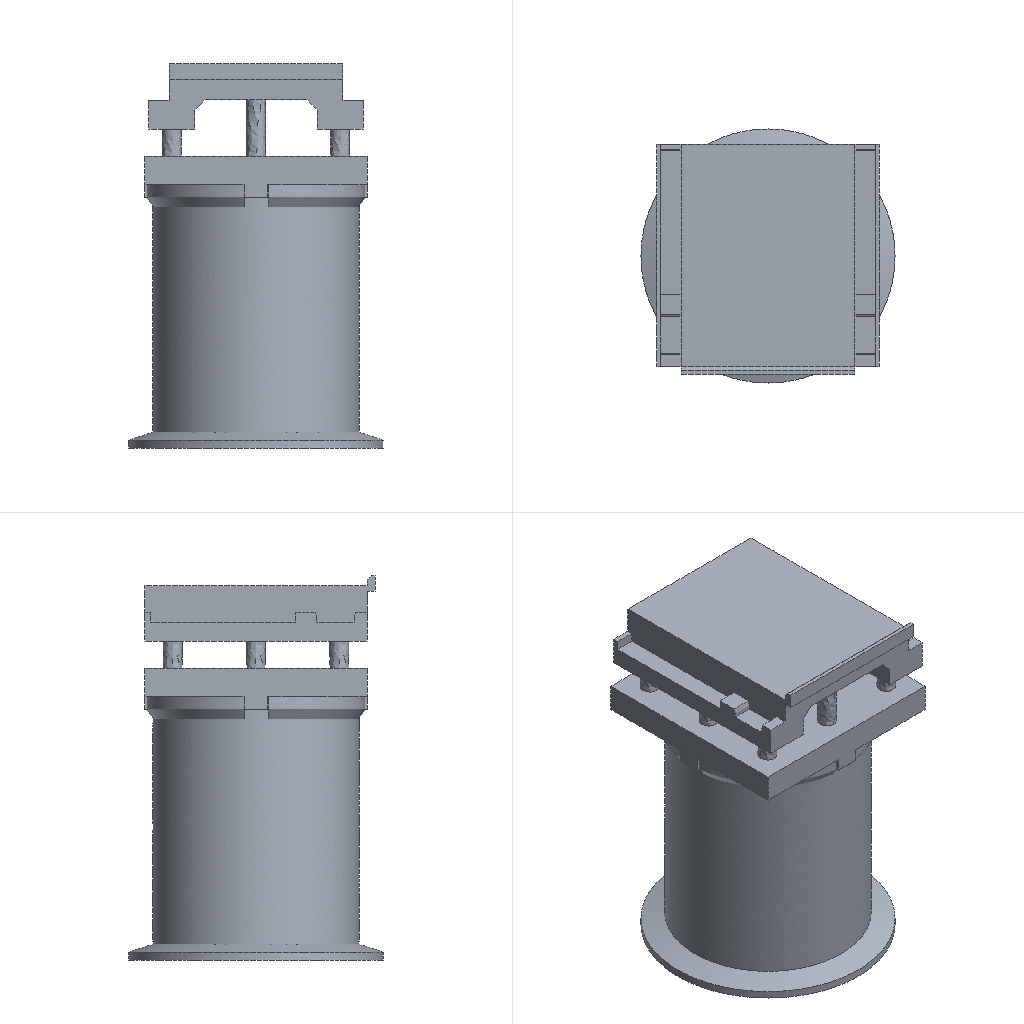Simulation study | ansys workbench
Ansys APDL input file, long lists of numbers shortened:
/batch
/config,noeldb,1     ! force off writing results to database
*get,_wallstrt,active,,time,wall
! ANSYS input file written by Workbench version 2022 R1
! File used for geometry attach:
/title,___--____ 2 (B5)
! ****** Begin Custom Load Command Snippet ******
/COM, ACT Extensions:
/COM,     LSDYNA, 2021.1
/COM,
! ****** End   Custom Load Command Snippet ******
*DIM,_wb_ProjectScratch_dir,string,248
_wb_ProjectScratch_dir(1) = ''
*DIM,_wb_SolverFiles_dir,string,248
_wb_SolverFiles_dir(1) = ''
*DIM,_wb_userfiles_dir,string,248
_wb_userfiles_dir(1) = ''
/com,--- Data in consistent MKS units. See Solving Units in the help system for more information.
/units,MKS
/nopr
/wb,file,start              !  signify a WB generated input file
/prep7
! Turn off shape checking because checks already performed inside WB mesher.
! See help system for more information.
SHPP,OFF,,NOWARN
/nolist
etcon,set             ! allow ANSYS to choose best KEYOP's for 180x elements, resets any applicable keyopt to MAPDL defaults
/com,*********** Nodes for the whole assembly ***********
nblock,3,,165333
(1i9,3e20.9e3)
        1    -4.091861413E+02     3.968814041E+01    -2.039000000E+01
! (150302 more lines like these left out)
-1
/wb,elem,start            !  set before creation of elements
/com,*********** Elements for Body 1 "a953f0-7" ***********
et,1,187
eblock,19,solid,,87505
(19i9)
        1        1        1        1        0        0        0        0       10        0        1    11820    23372    11975    23358    91085    91919    91082    91084
! (175009 more lines like these left out)
-1
/wb,elem,end               !  done creating elements
/com,*********** Send User Defined Coordinate System(s) ***********
csys,0
toffst,273.15,  ! Temperature offset from absolute zero
/com,*********** Set Reference Temperature ***********
tref,22.
/wb,mat,start              !  starting to send materials
/com,*********** Send Materials ***********
Temperature = 'TEMP' ! Temperature
MP,DENS,1,2300,	! kg m^-3
MP,ALPX,1,1.4e-05,	! C^-1
MP,C,1,780,	! J kg^-1 C^-1
MP,KXX,1,0.72,	! W m^-1 C^-1
MP,EX,1,30000000000,	! Pa
MP,NUXY,1,0.18,
/wb,mat,end                !  done sending materials
!************************* Model Summary ********************
!a953f0-7,	混凝土,	matid,	1
!************************* End Model Summary ********************
! get the diagonal of the bounding box. Needed later for other things
*get,_xmin,node,,mnloc,x
*get,_ymin,node,,mnloc,y
*get,_zmin,node,,mnloc,z
*get,_xmax,node,,mxloc,x
*get,_ymax,node,,mxloc,y
*get,_zmax,node,,mxloc,z
_ASMDIAG=(_xmax-_xmin)*(_xmax-_xmin)+(_ymax-_ymin)*(_ymax-_ymin)+(_zmax-_zmin)*(_zmax-_zmin)
_ASMDIAG=SQRT(_ASMDIAG)
/wb,contact,start          !  starting to send contact
/wb,contact,end            !  done creating contacts
/golist
/wb,load,start             !  starting to send loads
/com,*********** Fixed Supports ***********
CMBLOCK,_FIXEDSU,NODE,     7355
(8i10)
         1        96       121       122       123       124       125       126
! (919 more lines like these left out)
cmsel,s,_FIXEDSU
d,all,all
nsel,all
/com,*********** Define Force Using Surface Effect Elements ***********
local,12,0,0.,0.,0.,0.,0.,0.
csys,0
et,2,154
eblock,10,,,7449
(15i9)
   119600        2        2        2       12       15    11737       14       14    23478    23472       14    23468
! (7448 more lines like these left out)
-1
esel,s,type,,2
keyop,2,2,1                ! Apply load in local coordinate system
keyop,2,7,1                ! Use original area so load is constant in large deformation
esel,all
/gst,on,on
fini
*get,_numnode,node,0,count
*get,_numelem,elem,0,count
*get, _MAXELEMNUM, elem, 0, NUM, MAX
*get, _MAXNODENUM, node, 0, NUM, MAX
*get, _MAXELEMTYPE, etyp, 0, NUM, MAX
*get, _MAXREALCONST, real, 0, NUM, MAX
/go
/wb,load,end               !  done creating loads
/com,--- Number of total nodes = %_numnode%
/com,--- Number of contact elements = 7449
/com,--- Number of spring elements = 0
/com,--- Number of bearing elements = 0
/com,--- Number of solid elements = 87505
/com,--- Number of condensed parts = 0
/com,--- Number of total elements = %_numelem%
*get,_wallbsol,active,,time,wall
/com,****************************************************************************
/com,*************************    SOLUTION       ********************************
/com,****************************************************************************
/solu
antype,0                   ! static analysis
_thickRatio=  1     ! Ratio of thick parts in the model
eqsl,pcg,1e-8,,,,,,1
cntr,print,1               ! print out contact info and also make no initial contact an error
dmpoption,emat,no             ! Don't combine emat file for DANSYS
dmpoption,esav,no             ! Don't combine esav file for DANSYS
nldiag,cont,iter           ! print out contact info each equilibrium iteration
rescontrol,,none                 ! Do not keep any restart files
/com,****************************************************
/com,******************* SOLVE FOR LS 1 OF 1 ****************
esel,s,type,,2
nsle
sfe,all,1,pres,1,0.
sfe,all,2,pres,1,-859.904
sfe,all,3,pres,1,0.
nsel,all
esel,all
acel,0.,0.,9.807
/nopr
/gopr
nsub,1,1,1
time,1.
outres,erase
outres,all,none
outres,nsol,all,
outres,rsol,all
outres,eangl,all
outres,etmp,all
outres,veng,all
outres,strs,all,
outres,epel,all,
outres,eppl,all,
outres,cont,all,
! *********** WB SOLVE COMMAND ***********
! check interactive state
*get,ANSINTER_,active,,int
*if,ANSINTER_,ne,0,then
/eof
*endif
solve
/com *************** Write FE CONNECTORS *********
CEWRITE,file,ce,,INTE
/com,****************************************************
/com,*************** FINISHED SOLVE FOR LS 1 *************
*get,_wallasol,active,,time,wall
/nopr
*get,_numnode,node,0,count
*get,_numelem,elem,0,count
*get, _MAXELEMNUM, elem, 0, NUM, MAX
*get, _MAXNODENUM, node, 0, NUM, MAX,,,INTERNAL
*get, _MAXELEMTYPE, etyp, 0, NUM, MAX
*get, _MAXREALCONST, real, 0, NUM, MAX
/gopr
*get,_PCGITER,active,,solu,cgiter
/post1
xmlo,ENCODING,ISO-8859-1
xmlo,parm
/xml,parm,xml
fini
/gopr
*get,_walldone,active,,time,wall
_preptime=(_wallbsol-_wallstrt)*3600
_solvtime=(_wallasol-_wallbsol)*3600
_posttime=(_walldone-_wallasol)*3600
_totaltim=(_walldone-_wallstrt)*3600
*get,_dlbratio,active,0,solu,dlbr
*get,_combtime,active,0,solu,comb
*get,_ssmode,active,0,solu,ssmm
*get,_ndofs,active,0,solu,ndof
*get,_sol_end_time,active,0,set,time
*if,_sol_end_time,eq,1.,then
/fclean				!clean distributed files
*endif
/com,--- Total number of nodes = %_numnode%
/com,--- Total number of elements = %_numelem%
/com,--- Element load balance ratio = %_dlbratio%
/com,--- Time to combine distributed files = %_combtime%
/com,--- Sparse memory mode = %_ssmode%
/com,--- Number of DOF = %_ndofs%
/wb,file,end               ! done with WB generated input